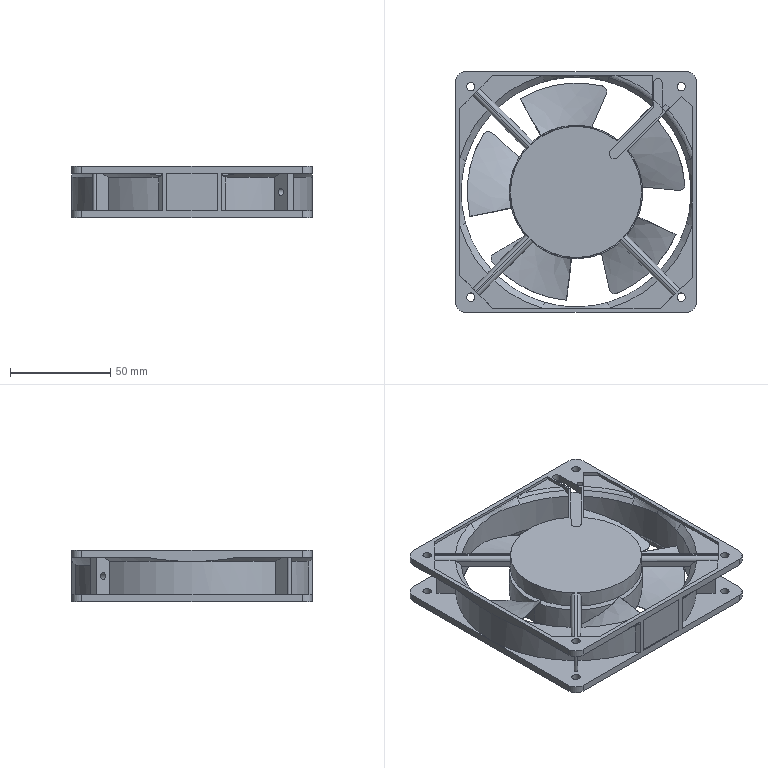Part | NX | features BREP 2 | 2 solids | 218 faces | box 120 x 120 x 25.5 mm | volume 116153 mm3 | plane 113 | spline 41 | cylinder 40 | cone 16 | torus 8 | commonest cylinder face diameters 4.2 x8 10 x8 120 x7 4 x6 1.8 x3 3.5 x2